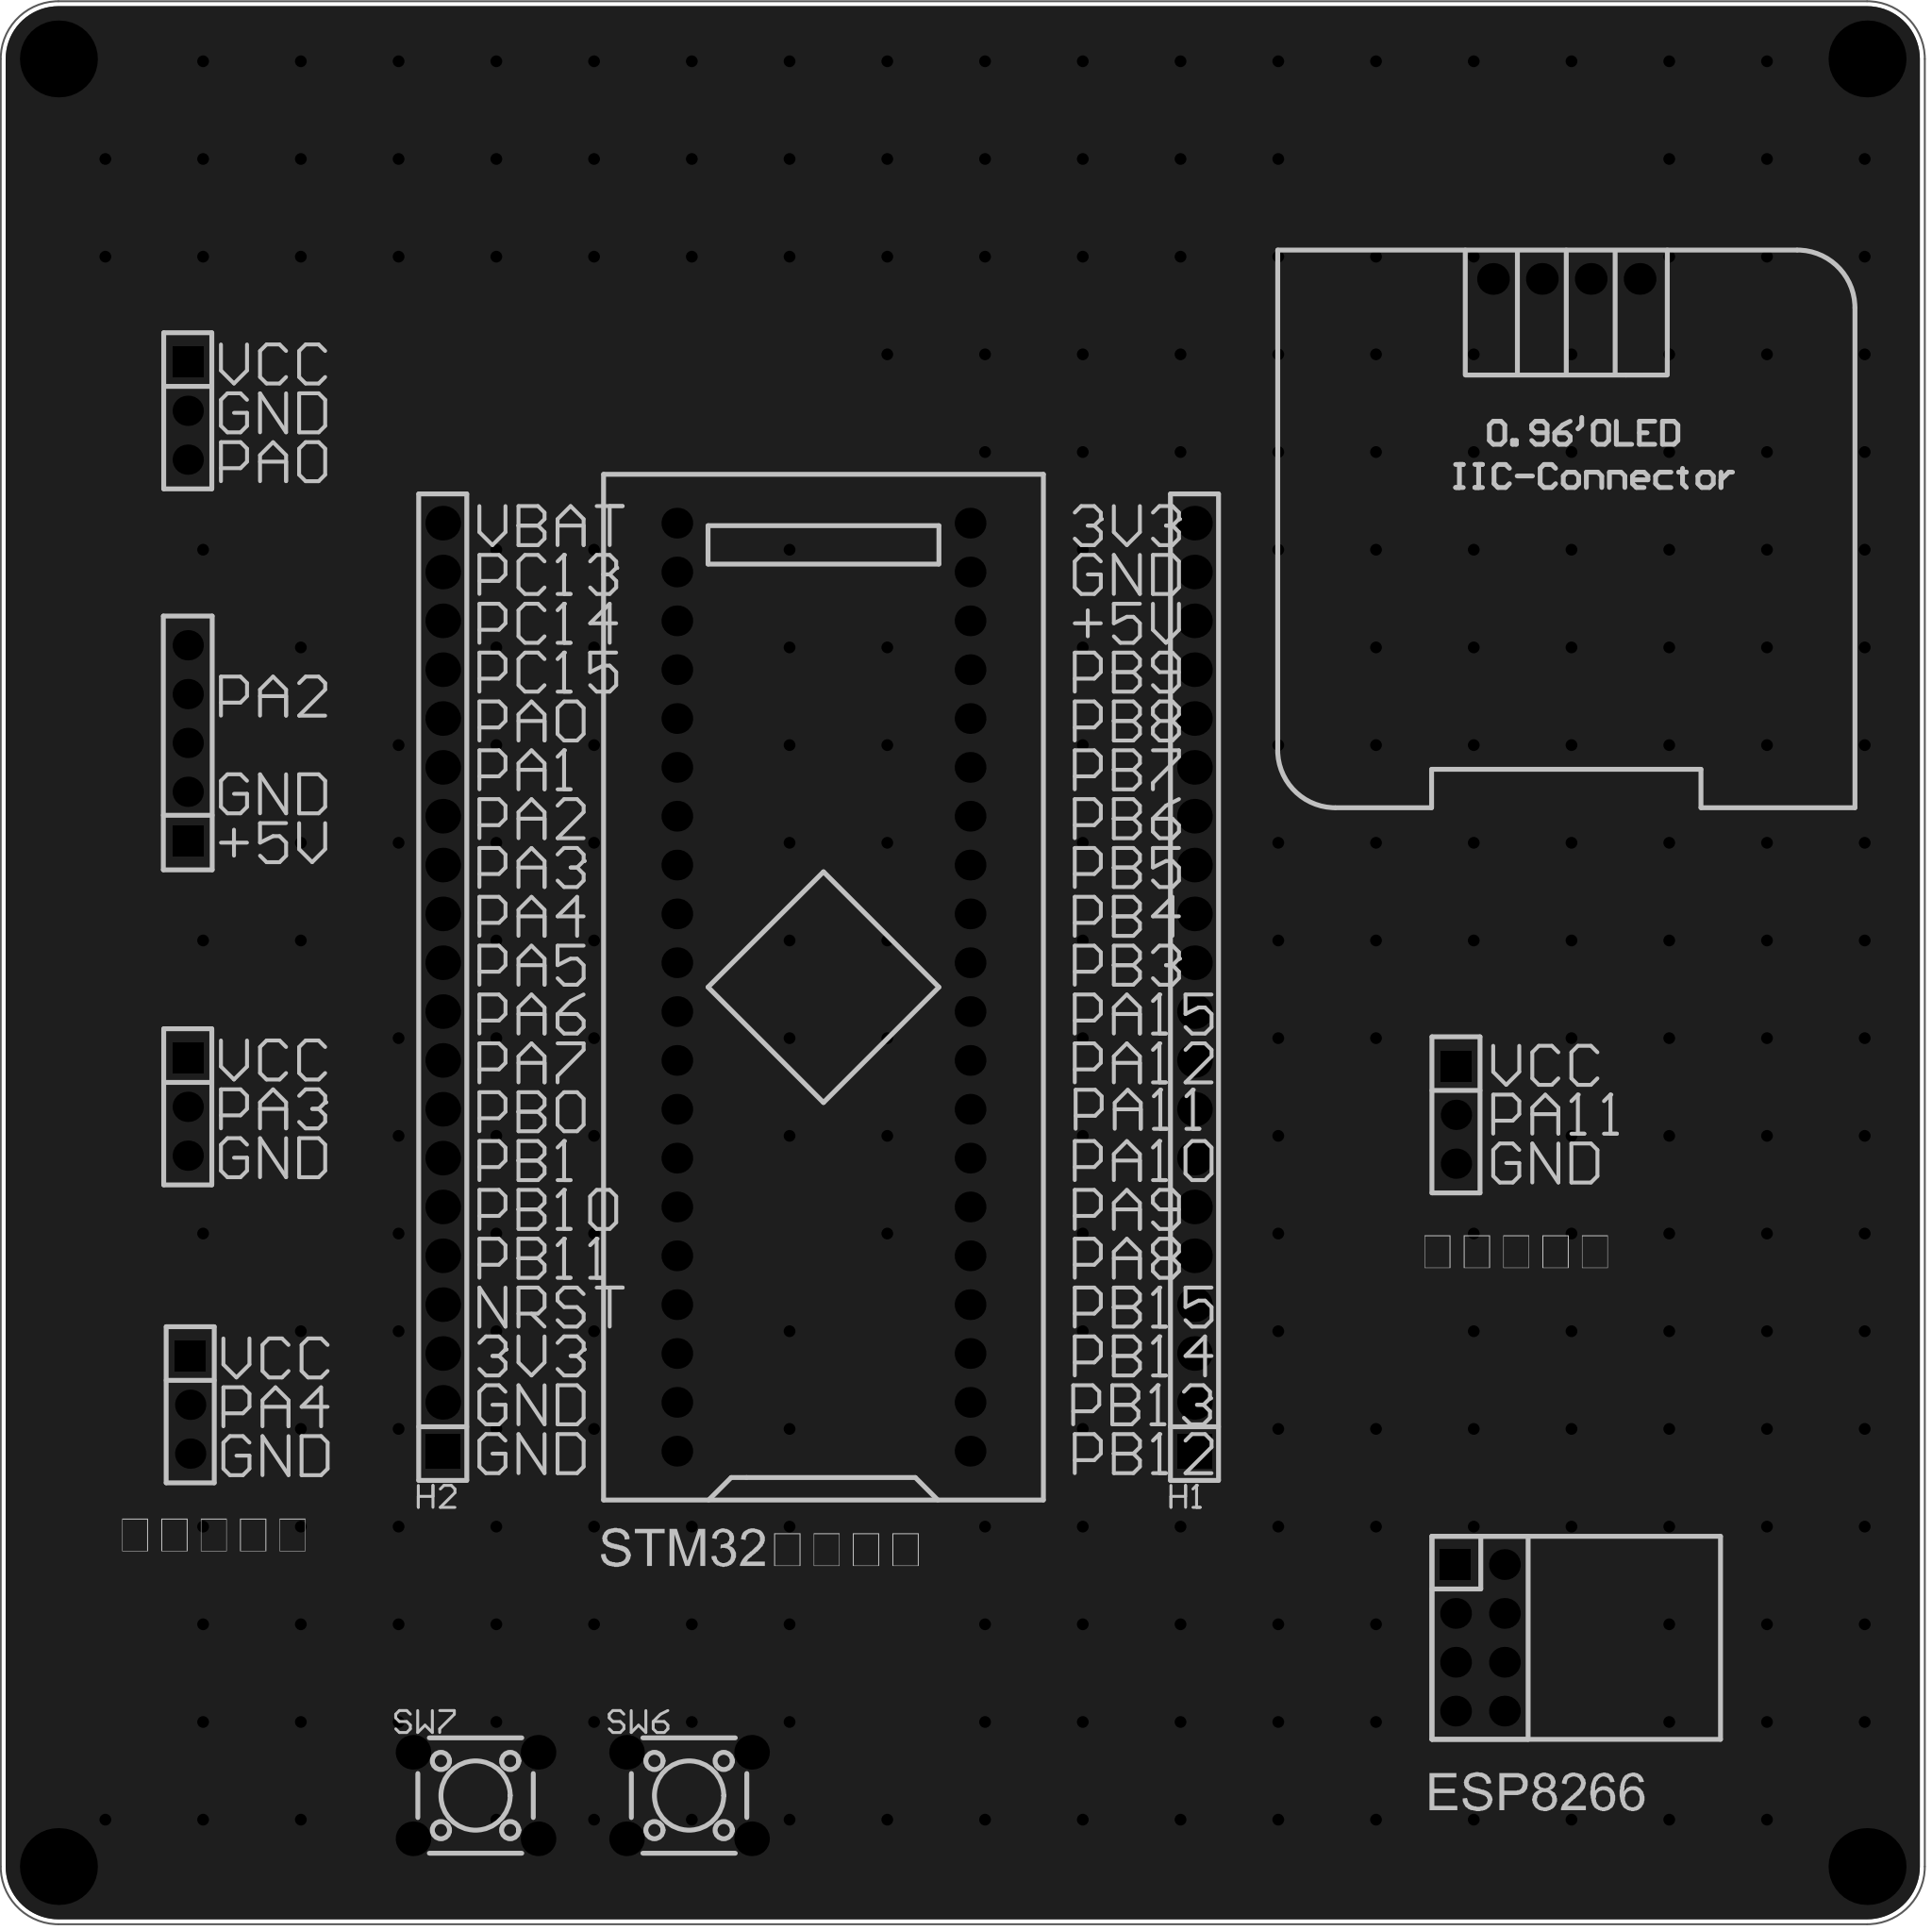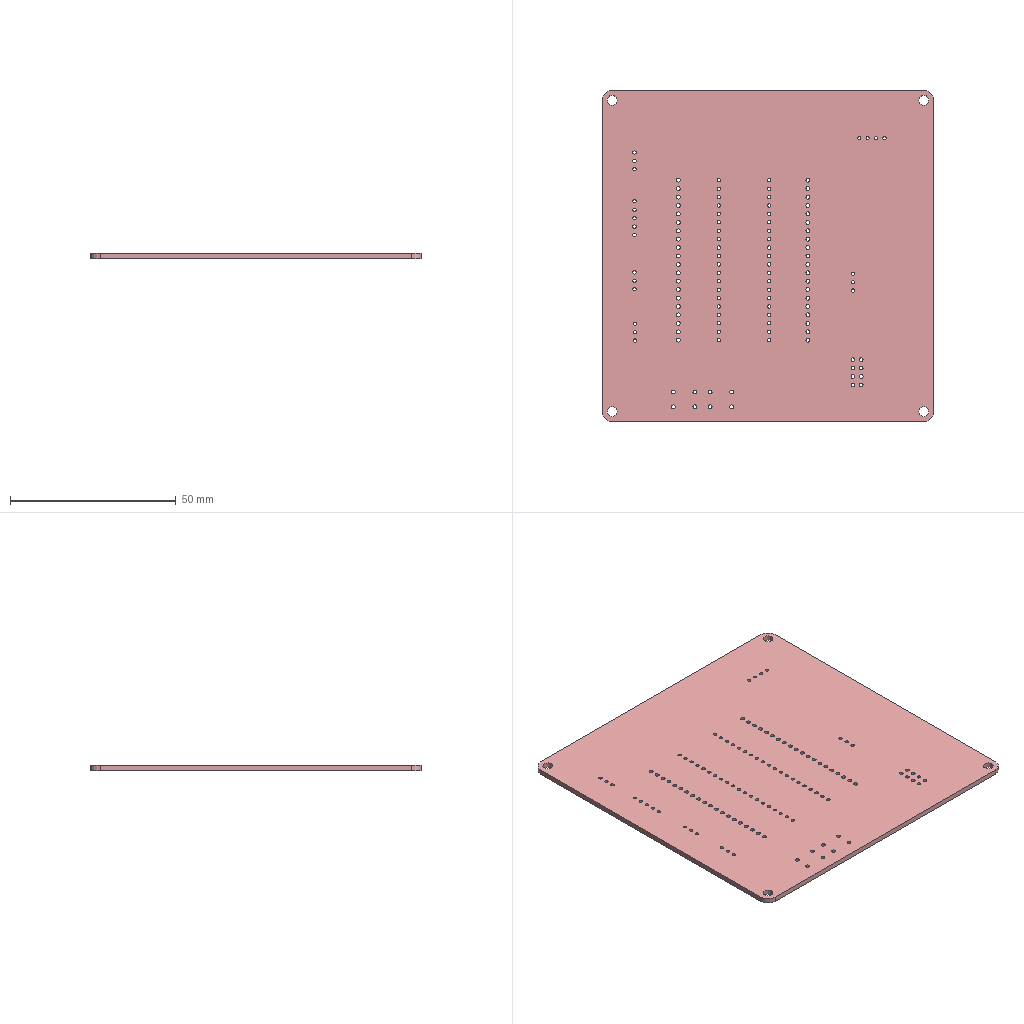Circuit board layout | Altium Designer | box 100 x 100 x 1.6 mm
Layer stack:
# Altium Designer layer stack of  (unit mm; dielectric type: 0 none, 1 core, 2 prepreg, 3 surface material)
index,name,kind,layer,copper_thickness_mm,dielectric_type,dielectric_thickness_mm,dielectric_material,dielectric_constant
0,Top Paste Mask Layer,other,,,,,,
1,Top Silkscreen Layer,other,,,,,,
2,Top Solder Mask Layer,dielectric,,,3,0.01,,3.3
3,Top Layer,copper,Top Layer,0.035,,,,
4,Dielectric1,dielectric,,,3,1.51,FR4,4.5
5,Bottom Layer,copper,Bottom Layer,0.035,,,,
6,Bottom Solder Mask Layer,dielectric,,,3,0.01,,3.3
7,Bottom Silkscreen Layer,other,,,,,,
8,Bottom Paste Mask Layer,other,,,,,,
# drill layer pairs: low layer,high layer
drill_pair,Top Layer,Bottom Layer
Part placement:
Designator,Comment,Layer,Footprint,Center-X(mm),Center-Y(mm),Rotation
U1,STM32F103C8T6-Card,TopLayer,CONN-TH_L53.3-W22.9_STM32F103C8T6-CARD,123.317,127.635,90
H22,,TopLayer,HDR-TH_3P-P2.54-V-F,90.277,157.607,270
OLED1,,TopLayer,0.96OLED_4P,161.925,164.465,0
H21,,TopLayer,HDR-TH_5P-P2.54-V-F,90.277,140.335,90
H15,,TopLayer,HDR-TH_3P-P2.54-V-F,90.277,121.412,270
H16,,TopLayer,HDR-TH_8P-P2.54-V-F-R2-C4-S2.54-1,157.44,93.799,270
H1,,TopLayer,HDR-TH_20P-P2.54-V-F,142.6,127.635,90
H2,,TopLayer,HDR-TH_20P-P2.54-V-F,103.529,127.635,90
H17,,TopLayer,HDR-TH_3P-P2.54-V-F,90.404,105.918,270
H18,,TopLayer,HDR-TH_3P-P2.54-V-F,156.19,120.995,270
SW6,,TopLayer,SW-TH_4P-L6.0-W6.0-P4.50-LS6.5,116.332,85.598,0
SW7,,TopLayer,SW-TH_4P-L6.0-W6.0-P4.50-LS6.5,105.235,85.598,0
Pad and via stacks:
# Altium Designer via and pad stacks of  (unit mm). Each distinct definition once, with the count of objects using it.
# via: kind,start_layer,end_layer,hole_mm,diameter_mm,mode(0 simple;1 top-mid-bottom;2 full stack),diameter_per_layer,count,example_net
# pad: kind,layer,hole_mm,hole_type(0 round;1 square;2 slot),plating,top_size,top_shape(1 round;2 rect;3 octagon;9 rounded rect),mid_size,bottom_size,mode,footprint,size_per_layer,count,example
pad,Multi-Layer,3,0,plated,4x4,1,4x4,4x4,0,,,4,1
pad,Multi-Layer,1,0,plated,1.6x1.6,1,1.6x1.6,1.6x1.6,0,CONN-TH_L53.3-W22.9_STM32F103C8T6-CARD,,40,U1.1
pad,Multi-Layer,1.02,0,plated,1.575x1.575,1,1.575x1.575,1.575x1.575,0,HDR-TH_3P-P2.54-V-F,,8,H22.3
pad,Multi-Layer,1.02,0,plated,1.575x1.575,2,1.575x1.575,1.575x1.575,0,HDR-TH_3P-P2.54-V-F,,4,H22.1
pad,Multi-Layer,1,0,plated,1.65x1.65,1,1.65x1.65,1.65x1.65,0,0.96OLED_4P,,4,OLED1.4
pad,Multi-Layer,1.02,0,plated,1.575x1.575,1,1.575x1.575,1.575x1.575,0,HDR-TH_5P-P2.54-V-F,,4,H21.5
pad,Multi-Layer,1.02,0,plated,1.575x1.575,2,1.575x1.575,1.575x1.575,0,HDR-TH_5P-P2.54-V-F,,1,H21.1
pad,Multi-Layer,1.1,0,plated,1.6x1.6,2,1.6x1.6,1.6x1.6,0,HDR-TH_8P-P2.54-V-F-R2-C4-S2.54-1,,1,H16.1
pad,Multi-Layer,1.1,0,plated,1.6x1.6,1,1.6x1.6,1.6x1.6,0,HDR-TH_8P-P2.54-V-F-R2-C4-S2.54-1,,7,H16.2
pad,Multi-Layer,1.2,0,plated,1.8x1.8,2,1.8x1.8,1.8x1.8,0,HDR-TH_20P-P2.54-V-F,,2,H1.1
pad,Multi-Layer,1.2,0,plated,1.8x1.8,1,1.8x1.8,1.8x1.8,0,HDR-TH_20P-P2.54-V-F,,38,H1.2
pad,Multi-Layer,1.2,0,plated,1.8x1.8,1,1.8x1.8,1.8x1.8,0,SW-TH_4P-L6.0-W6.0-P4.50-LS6.5,,8,SW6.1
via,Top Layer,Bottom Layer,0.3048,0.61,0,,261,GND
Copper pours:
name,layer,net,type(0 solid;1 hatched;2 none)
Bottom Layer-GND,Bottom Layer,GND,0
Top Layer-GND,Top Layer,GND,0